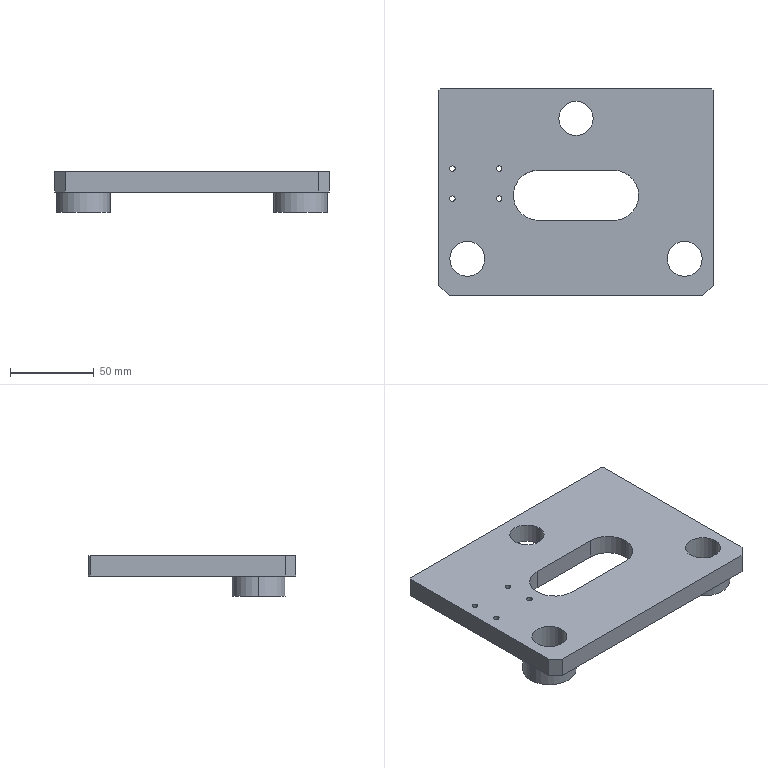Part | STEP file | support plate 32 | 1 solid | 51 faces | box 164 x 124 x 24 mm | volume 216301 mm3 | cylinder 29 | plane 14 | cone 8 | commonest cylinder face diameters 3.3 x8 4.2 x8 21 x4 32 x4 30 x3 20.5 x2